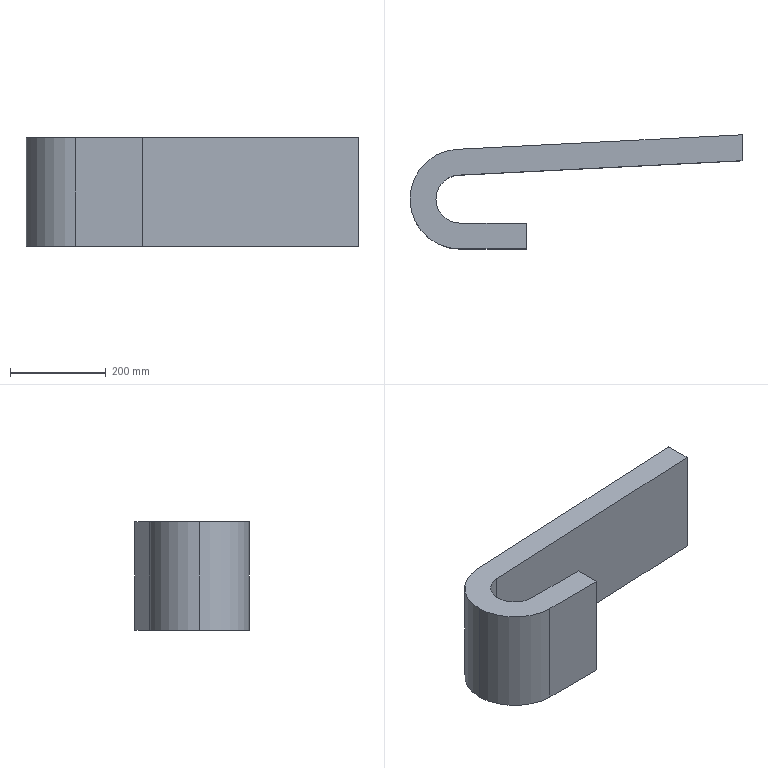Part | STEP file | TKR26H40W200R75+37L-FU-MU-Part-1 | 1 solid | 24 faces | box 692.25 x 238 x 226 mm | volume 4074377 mm3 | plane 16 | cylinder 8 | commonest cylinder face diameters 100 x2 114 x2 194 x2 208 x2